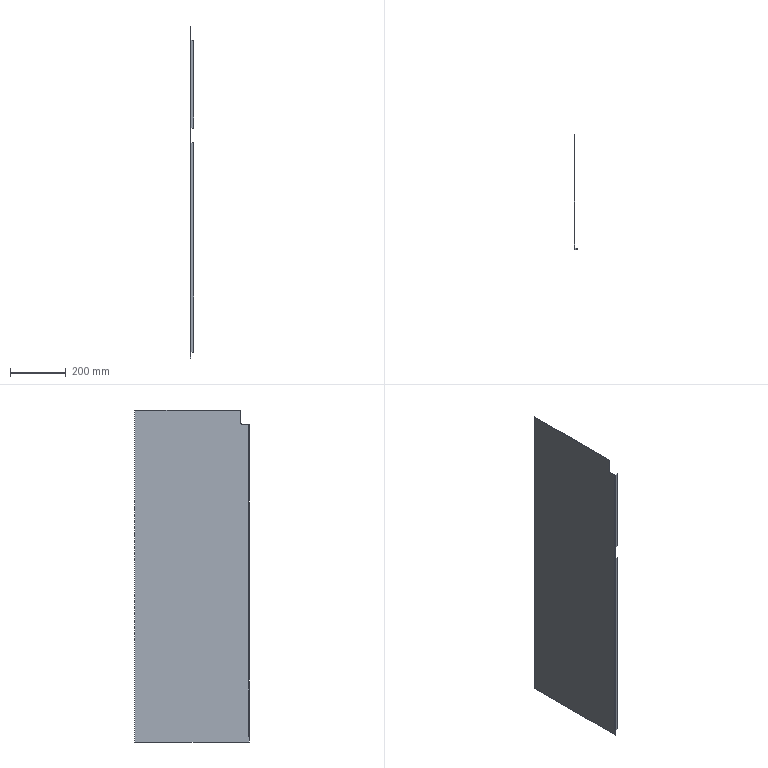Part | SolidWorks | 1 solid | 28 faces | box 12 x 410 x 1188 mm | volume 991648 mm3 | plane 25 | cylinder 3 | commonest cylinder face diameters 0.2 x1 4.2 x1 10 x1
STEP:
#1=CARTESIAN_POINT('',(10.,-205.,-573.25));
#2=VERTEX_POINT('',#1);
#3=CARTESIAN_POINT('',(10.,-205.,176.75));
#4=VERTEX_POINT('',#3);
#5=CARTESIAN_POINT('',(10.,-205.,0.));
#6=DIRECTION('',(0.,0.,1.));
#7=VECTOR('',#6,1000.);
#8=LINE('',#5,#7);
#9=EDGE_CURVE('',#2,#4,#8,.T.);
#10=ORIENTED_EDGE('',*,*,#9,.T.);
#11=CARTESIAN_POINT('',(0.1,-205.,176.75));
#12=VERTEX_POINT('',#11);
#13=CARTESIAN_POINT('',(0.,-205.,176.75));
#14=DIRECTION('',(1.,0.,0.));
#15=VECTOR('',#14,1000.);
#16=LINE('',#13,#15);
#17=EDGE_CURVE('',#12,#4,#16,.T.);
#18=ORIENTED_EDGE('',*,*,#17,.F.);
#19=CARTESIAN_POINT('',(0.1,-205.,-573.25));
#20=VERTEX_POINT('',#19);
#21=CARTESIAN_POINT('',(0.1,-205.,543.25));
#22=DIRECTION('',(0.,0.,1.));
#23=VECTOR('',#22,1000.);
#24=LINE('',#21,#23);
#25=EDGE_CURVE('',#20,#12,#24,.T.);
#26=ORIENTED_EDGE('',*,*,#25,.F.);
#27=CARTESIAN_POINT('',(0.,-205.,-573.25));
#28=DIRECTION('',(1.,0.,0.));
#29=VECTOR('',#28,1000.);
#30=LINE('',#27,#29);
#31=EDGE_CURVE('',#20,#2,#30,.T.);
#32=ORIENTED_EDGE('',*,*,#31,.T.);
#33=EDGE_LOOP('',(#10,#18,#26,#32));
#34=FACE_OUTER_BOUND('',#33,.T.);
#35=CARTESIAN_POINT('',(0.,-205.,0.));
#36=DIRECTION('',(0.,1.,0.));
#37=DIRECTION('',(-1.,0.,0.));
#38=AXIS2_PLACEMENT_3D('',#35,#36,#37);
#39=PLANE('',#38);
#40=ADVANCED_FACE('',(#34),#39,.F.);
#41=CARTESIAN_POINT('',(10.,-203.,176.75));
#42=VERTEX_POINT('',#41);
#43=CARTESIAN_POINT('',(0.1,-203.,176.75));
#44=VERTEX_POINT('',#43);
#45=CARTESIAN_POINT('',(0.,-203.,176.75));
#46=DIRECTION('',(-1.,0.,0.));
#47=VECTOR('',#46,1000.);
#48=LINE('',#45,#47);
#49=EDGE_CURVE('',#42,#44,#48,.T.);
#50=ORIENTED_EDGE('',*,*,#49,.F.);
#51=CARTESIAN_POINT('',(10.,-203.,-573.25));
#52=VERTEX_POINT('',#51);
#53=CARTESIAN_POINT('',(10.,-203.,543.25));
#54=DIRECTION('',(0.,0.,1.));
#55=VECTOR('',#54,1000.);
#56=LINE('',#53,#55);
#57=EDGE_CURVE('',#52,#42,#56,.T.);
#58=ORIENTED_EDGE('',*,*,#57,.F.);
#59=CARTESIAN_POINT('',(0.1,-203.,-573.25));
#60=VERTEX_POINT('',#59);
#61=CARTESIAN_POINT('',(10.,-203.,-573.25));
#62=DIRECTION('',(1.,0.,0.));
#63=VECTOR('',#62,1000.);
#64=LINE('',#61,#63);
#65=EDGE_CURVE('',#60,#52,#64,.T.);
#66=ORIENTED_EDGE('',*,*,#65,.F.);
#67=CARTESIAN_POINT('',(0.1,-203.,543.25));
#68=DIRECTION('',(0.,0.,-1.));
#69=VECTOR('',#68,1000.);
#70=LINE('',#67,#69);
#71=EDGE_CURVE('',#44,#60,#70,.T.);
#72=ORIENTED_EDGE('',*,*,#71,.F.);
#73=EDGE_LOOP('',(#50,#58,#66,#72));
#74=FACE_OUTER_BOUND('',#73,.T.);
#75=CARTESIAN_POINT('',(0.,-203.,0.));
#76=DIRECTION('',(0.,1.,0.));
#77=DIRECTION('',(-1.,0.,0.));
#78=AXIS2_PLACEMENT_3D('',#75,#76,#77);
#79=PLANE('',#78);
#80=ADVANCED_FACE('',(#74),#79,.T.);
#81=ORIENTED_EDGE('',*,*,#57,.T.);
#82=CARTESIAN_POINT('',(10.,-205.001,176.75));
#83=DIRECTION('',(0.,1.,0.));
#84=VECTOR('',#83,1000.);
#85=LINE('',#82,#84);
#86=EDGE_CURVE('',#4,#42,#85,.T.);
#87=ORIENTED_EDGE('',*,*,#86,.F.);
#88=ORIENTED_EDGE('',*,*,#9,.F.);
#89=CARTESIAN_POINT('',(10.,-205.,-573.25));
#90=DIRECTION('',(0.,1.,0.));
#91=VECTOR('',#90,1000.);
#92=LINE('',#89,#91);
#93=EDGE_CURVE('',#2,#52,#92,.T.);
#94=ORIENTED_EDGE('',*,*,#93,.T.);
#95=EDGE_LOOP('',(#81,#87,#88,#94));
#96=FACE_OUTER_BOUND('',#95,.T.);
#97=CARTESIAN_POINT('',(10.,-205.,543.25));
#98=DIRECTION('',(-1.,0.,0.));
#99=DIRECTION('',(0.,-1.,0.));
#100=AXIS2_PLACEMENT_3D('',#97,#98,#99);
#101=PLANE('',#100);
#102=ADVANCED_FACE('',(#96),#101,.F.);
#103=CARTESIAN_POINT('',(0.,-205.,-574.25));
#104=VERTEX_POINT('',#103);
#105=CARTESIAN_POINT('',(0.,-205.,-594.25));
#106=VERTEX_POINT('',#105);
#107=CARTESIAN_POINT('',(0.,-205.,-594.25));
#108=DIRECTION('',(0.,0.,-1.));
#109=VECTOR('',#108,1000.);
#110=LINE('',#107,#109);
#111=EDGE_CURVE('',#104,#106,#110,.T.);
#112=ORIENTED_EDGE('',*,*,#111,.F.);
#113=CARTESIAN_POINT('',(-2.,-205.,-574.25));
#114=VERTEX_POINT('',#113);
#115=CARTESIAN_POINT('',(0.,-205.,-574.25));
#116=DIRECTION('',(-1.,0.,0.));
#117=VECTOR('',#116,1000.);
#118=LINE('',#115,#117);
#119=EDGE_CURVE('',#104,#114,#118,.T.);
#120=ORIENTED_EDGE('',*,*,#119,.T.);
#121=CARTESIAN_POINT('',(-2.,-205.,-594.25));
#122=VERTEX_POINT('',#121);
#123=CARTESIAN_POINT('',(-2.,-205.,-594.25));
#124=DIRECTION('',(0.,0.,-1.));
#125=VECTOR('',#124,1000.);
#126=LINE('',#123,#125);
#127=EDGE_CURVE('',#114,#122,#126,.T.);
#128=ORIENTED_EDGE('',*,*,#127,.T.);
#129=CARTESIAN_POINT('',(-2.,-205.,-594.25));
#130=DIRECTION('',(1.,0.,0.));
#131=VECTOR('',#130,1000.);
#132=LINE('',#129,#131);
#133=EDGE_CURVE('',#122,#106,#132,.T.);
#134=ORIENTED_EDGE('',*,*,#133,.T.);
#135=EDGE_LOOP('',(#112,#120,#128,#134));
#136=FACE_OUTER_BOUND('',#135,.T.);
#137=CARTESIAN_POINT('',(-2.,-205.,-594.25));
#138=DIRECTION('',(0.,-1.,0.));
#139=DIRECTION('',(0.,0.,-1.));
#140=AXIS2_PLACEMENT_3D('',#137,#138,#139);
#141=PLANE('',#140);
#142=ADVANCED_FACE('',(#136),#141,.T.);
#143=CARTESIAN_POINT('',(-2.,-179.,543.25));
#144=VERTEX_POINT('',#143);
#145=CARTESIAN_POINT('',(-2.,-202.9,543.25));
#146=VERTEX_POINT('',#145);
#147=CARTESIAN_POINT('',(-2.,0.,543.25));
#148=DIRECTION('',(0.,-1.,0.));
#149=VECTOR('',#148,1000.);
#150=LINE('',#147,#149);
#151=EDGE_CURVE('',#144,#146,#150,.T.);
#152=ORIENTED_EDGE('',*,*,#151,.F.);
#153=CARTESIAN_POINT('',(-2.,-174.,548.25));
#154=VERTEX_POINT('',#153);
#155=CARTESIAN_POINT('',(-2.,-179.,548.25));
#156=DIRECTION('',(-1.,0.,0.));
#157=DIRECTION('',(0.,0.,-1.));
#158=AXIS2_PLACEMENT_3D('',#155,#156,#157);
#159=CIRCLE('',#158,5.);
#160=EDGE_CURVE('',#154,#144,#159,.T.);
#161=ORIENTED_EDGE('',*,*,#160,.F.);
#162=CARTESIAN_POINT('',(-2.,-174.,594.25));
#163=VERTEX_POINT('',#162);
#164=CARTESIAN_POINT('',(-2.,-174.,598.25));
#165=DIRECTION('',(0.,0.,-1.));
#166=VECTOR('',#165,1000.);
#167=LINE('',#164,#166);
#168=EDGE_CURVE('',#163,#154,#167,.T.);
#169=ORIENTED_EDGE('',*,*,#168,.F.);
#170=CARTESIAN_POINT('',(-2.,205.,594.25));
#171=VERTEX_POINT('',#170);
#172=CARTESIAN_POINT('',(-2.,-205.,594.25));
#173=DIRECTION('',(0.,-1.,0.));
#174=VECTOR('',#173,1000.);
#175=LINE('',#172,#174);
#176=EDGE_CURVE('',#171,#163,#175,.T.);
#177=ORIENTED_EDGE('',*,*,#176,.F.);
#178=CARTESIAN_POINT('',(-2.,205.,-594.25));
#179=VERTEX_POINT('',#178);
#180=CARTESIAN_POINT('',(-2.,205.,-594.25));
#181=DIRECTION('',(0.,0.,1.));
#182=VECTOR('',#181,1000.);
#183=LINE('',#180,#182);
#184=EDGE_CURVE('',#179,#171,#183,.T.);
#185=ORIENTED_EDGE('',*,*,#184,.F.);
#186=CARTESIAN_POINT('',(-2.,-205.,-594.25));
#187=DIRECTION('',(0.,1.,0.));
#188=VECTOR('',#187,1000.);
#189=LINE('',#186,#188);
#190=EDGE_CURVE('',#122,#179,#189,.T.);
#191=ORIENTED_EDGE('',*,*,#190,.F.);
#192=ORIENTED_EDGE('',*,*,#127,.F.);
#193=CARTESIAN_POINT('',(-2.,-201.9,-574.25));
#194=VERTEX_POINT('',#193);
#195=CARTESIAN_POINT('',(-2.,0.,-574.25));
#196=DIRECTION('',(0.,-1.,0.));
#197=VECTOR('',#196,1000.);
#198=LINE('',#195,#197);
#199=EDGE_CURVE('',#194,#114,#198,.T.);
#200=ORIENTED_EDGE('',*,*,#199,.F.);
#201=CARTESIAN_POINT('',(-2.,-201.9,-573.25));
#202=VERTEX_POINT('',#201);
#203=CARTESIAN_POINT('',(-2.,-201.9,0.));
#204=DIRECTION('',(0.,0.,-1.));
#205=VECTOR('',#204,1000.);
#206=LINE('',#203,#205);
#207=EDGE_CURVE('',#202,#194,#206,.T.);
#208=ORIENTED_EDGE('',*,*,#207,.F.);
#209=CARTESIAN_POINT('',(-2.,-202.9,-573.25));
#210=VERTEX_POINT('',#209);
#211=CARTESIAN_POINT('',(-2.,0.,-573.25));
#212=DIRECTION('',(0.,1.,0.));
#213=VECTOR('',#212,1000.);
#214=LINE('',#211,#213);
#215=EDGE_CURVE('',#210,#202,#214,.T.);
#216=ORIENTED_EDGE('',*,*,#215,.F.);
#217=CARTESIAN_POINT('',(-2.,-202.9,-573.25));
#218=DIRECTION('',(0.,0.,1.));
#219=VECTOR('',#218,1000.);
#220=LINE('',#217,#219);
#221=EDGE_CURVE('',#210,#146,#220,.T.);
#222=ORIENTED_EDGE('',*,*,#221,.T.);
#223=EDGE_LOOP('',(#152,#161,#169,#177,#185,#191,#192,#200,#208,#216,#222));
#224=FACE_OUTER_BOUND('',#223,.T.);
#225=CARTESIAN_POINT('',(-2.,0.,0.));
#226=DIRECTION('',(1.,0.,0.));
#227=DIRECTION('',(0.,0.,-1.));
#228=AXIS2_PLACEMENT_3D('',#225,#226,#227);
#229=PLANE('',#228);
#230=ADVANCED_FACE('',(#224),#229,.F.);
#231=CARTESIAN_POINT('',(0.,-174.,548.25));
#232=VERTEX_POINT('',#231);
#233=CARTESIAN_POINT('',(0.,-179.,543.25));
#234=VERTEX_POINT('',#233);
#235=CARTESIAN_POINT('',(0.,-179.,548.25));
#236=DIRECTION('',(-1.,0.,0.));
#237=DIRECTION('',(0.,0.,-1.));
#238=AXIS2_PLACEMENT_3D('',#235,#236,#237);
#239=CIRCLE('',#238,5.);
#240=EDGE_CURVE('',#232,#234,#239,.T.);
#241=ORIENTED_EDGE('',*,*,#240,.T.);
#242=CARTESIAN_POINT('',(0.,-202.9,543.25));
#243=VERTEX_POINT('',#242);
#244=CARTESIAN_POINT('',(0.,-202.9,543.25));
#245=DIRECTION('',(0.,1.,0.));
#246=VECTOR('',#245,1000.);
#247=LINE('',#244,#246);
#248=EDGE_CURVE('',#243,#234,#247,.T.);
#249=ORIENTED_EDGE('',*,*,#248,.F.);
#250=CARTESIAN_POINT('',(0.,-202.9,-573.25));
#251=VERTEX_POINT('',#250);
#252=CARTESIAN_POINT('',(0.,-202.9,-573.25));
#253=DIRECTION('',(0.,0.,1.));
#254=VECTOR('',#253,1000.);
#255=LINE('',#252,#254);
#256=EDGE_CURVE('',#251,#243,#255,.T.);
#257=ORIENTED_EDGE('',*,*,#256,.F.);
#258=CARTESIAN_POINT('',(0.,-201.9,-573.25));
#259=VERTEX_POINT('',#258);
#260=CARTESIAN_POINT('',(0.,-201.9,-573.25));
#261=DIRECTION('',(0.,-1.,0.));
#262=VECTOR('',#261,1000.);
#263=LINE('',#260,#262);
#264=EDGE_CURVE('',#259,#251,#263,.T.);
#265=ORIENTED_EDGE('',*,*,#264,.F.);
#266=CARTESIAN_POINT('',(0.,-201.9,-574.25));
#267=VERTEX_POINT('',#266);
#268=CARTESIAN_POINT('',(0.,-201.9,-574.25));
#269=DIRECTION('',(0.,0.,1.));
#270=VECTOR('',#269,1000.);
#271=LINE('',#268,#270);
#272=EDGE_CURVE('',#267,#259,#271,.T.);
#273=ORIENTED_EDGE('',*,*,#272,.F.);
#274=CARTESIAN_POINT('',(0.,-205.,-574.25));
#275=DIRECTION('',(0.,1.,0.));
#276=VECTOR('',#275,1000.);
#277=LINE('',#274,#276);
#278=EDGE_CURVE('',#104,#267,#277,.T.);
#279=ORIENTED_EDGE('',*,*,#278,.F.);
#280=ORIENTED_EDGE('',*,*,#111,.T.);
#281=CARTESIAN_POINT('',(0.,205.,-594.25));
#282=VERTEX_POINT('',#281);
#283=CARTESIAN_POINT('',(0.,-205.,-594.25));
#284=DIRECTION('',(0.,1.,0.));
#285=VECTOR('',#284,1000.);
#286=LINE('',#283,#285);
#287=EDGE_CURVE('',#106,#282,#286,.T.);
#288=ORIENTED_EDGE('',*,*,#287,.T.);
#289=CARTESIAN_POINT('',(0.,205.,594.25));
#290=VERTEX_POINT('',#289);
#291=CARTESIAN_POINT('',(0.,205.,-594.25));
#292=DIRECTION('',(0.,0.,1.));
#293=VECTOR('',#292,1000.);
#294=LINE('',#291,#293);
#295=EDGE_CURVE('',#282,#290,#294,.T.);
#296=ORIENTED_EDGE('',*,*,#295,.T.);
#297=CARTESIAN_POINT('',(0.,-174.,594.25));
#298=VERTEX_POINT('',#297);
#299=CARTESIAN_POINT('',(0.,-205.,594.25));
#300=DIRECTION('',(0.,-1.,0.));
#301=VECTOR('',#300,1000.);
#302=LINE('',#299,#301);
#303=EDGE_CURVE('',#290,#298,#302,.T.);
#304=ORIENTED_EDGE('',*,*,#303,.T.);
#305=CARTESIAN_POINT('',(0.,-174.,598.25));
#306=DIRECTION('',(0.,0.,-1.));
#307=VECTOR('',#306,1000.);
#308=LINE('',#305,#307);
#309=EDGE_CURVE('',#298,#232,#308,.T.);
#310=ORIENTED_EDGE('',*,*,#309,.T.);
#311=EDGE_LOOP('',(#241,#249,#257,#265,#273,#279,#280,#288,#296,#304,#310));
#312=FACE_OUTER_BOUND('',#311,.T.);
#313=CARTESIAN_POINT('',(0.,0.,0.));
#314=DIRECTION('',(1.,0.,0.));
#315=DIRECTION('',(0.,0.,-1.));
#316=AXIS2_PLACEMENT_3D('',#313,#314,#315);
#317=PLANE('',#316);
#318=ADVANCED_FACE('',(#312),#317,.T.);
#319=CARTESIAN_POINT('',(10.001,-174.,594.25));
#320=DIRECTION('',(1.,0.,0.));
#321=VECTOR('',#320,1000.);
#322=LINE('',#319,#321);
#323=EDGE_CURVE('',#163,#298,#322,.T.);
#324=ORIENTED_EDGE('',*,*,#323,.T.);
#325=ORIENTED_EDGE('',*,*,#303,.F.);
#326=CARTESIAN_POINT('',(-2.,205.,594.25));
#327=DIRECTION('',(1.,0.,0.));
#328=VECTOR('',#327,1000.);
#329=LINE('',#326,#328);
#330=EDGE_CURVE('',#171,#290,#329,.T.);
#331=ORIENTED_EDGE('',*,*,#330,.F.);
#332=ORIENTED_EDGE('',*,*,#176,.T.);
#333=EDGE_LOOP('',(#324,#325,#331,#332));
#334=FACE_OUTER_BOUND('',#333,.T.);
#335=CARTESIAN_POINT('',(-2.,-205.,594.25));
#336=DIRECTION('',(0.,0.,1.));
#337=DIRECTION('',(1.,0.,0.));
#338=AXIS2_PLACEMENT_3D('',#335,#336,#337);
#339=PLANE('',#338);
#340=ADVANCED_FACE('',(#334),#339,.T.);
#341=ORIENTED_EDGE('',*,*,#295,.F.);
#342=CARTESIAN_POINT('',(-2.,205.,-594.25));
#343=DIRECTION('',(1.,0.,0.));
#344=VECTOR('',#343,1000.);
#345=LINE('',#342,#344);
#346=EDGE_CURVE('',#179,#282,#345,.T.);
#347=ORIENTED_EDGE('',*,*,#346,.F.);
#348=ORIENTED_EDGE('',*,*,#184,.T.);
#349=ORIENTED_EDGE('',*,*,#330,.T.);
#350=EDGE_LOOP('',(#341,#347,#348,#349));
#351=FACE_OUTER_BOUND('',#350,.T.);
#352=CARTESIAN_POINT('',(-2.,205.,-594.25));
#353=DIRECTION('',(0.,1.,0.));
#354=DIRECTION('',(0.,0.,1.));
#355=AXIS2_PLACEMENT_3D('',#352,#353,#354);
#356=PLANE('',#355);
#357=ADVANCED_FACE('',(#351),#356,.T.);
#358=ORIENTED_EDGE('',*,*,#287,.F.);
#359=ORIENTED_EDGE('',*,*,#133,.F.);
#360=ORIENTED_EDGE('',*,*,#190,.T.);
#361=ORIENTED_EDGE('',*,*,#346,.T.);
#362=EDGE_LOOP('',(#358,#359,#360,#361));
#363=FACE_OUTER_BOUND('',#362,.T.);
#364=CARTESIAN_POINT('',(-2.,-205.,-594.25));
#365=DIRECTION('',(0.,0.,-1.));
#366=DIRECTION('',(-1.,0.,0.));
#367=AXIS2_PLACEMENT_3D('',#364,#365,#366);
#368=PLANE('',#367);
#369=ADVANCED_FACE('',(#363),#368,.T.);
#370=CARTESIAN_POINT('',(0.,-201.9,-574.25));
#371=DIRECTION('',(-1.,0.,0.));
#372=VECTOR('',#371,1000.);
#373=LINE('',#370,#372);
#374=EDGE_CURVE('',#267,#194,#373,.T.);
#375=ORIENTED_EDGE('',*,*,#374,.T.);
#376=ORIENTED_EDGE('',*,*,#199,.T.);
#377=ORIENTED_EDGE('',*,*,#119,.F.);
#378=ORIENTED_EDGE('',*,*,#278,.T.);
#379=EDGE_LOOP('',(#375,#376,#377,#378));
#380=FACE_OUTER_BOUND('',#379,.T.);
#381=CARTESIAN_POINT('',(0.,-205.,-574.25));
#382=DIRECTION('',(0.,0.,1.));
#383=DIRECTION('',(1.,0.,0.));
#384=AXIS2_PLACEMENT_3D('',#381,#382,#383);
#385=PLANE('',#384);
#386=ADVANCED_FACE('',(#380),#385,.T.);
#387=CARTESIAN_POINT('',(0.,-201.9,-573.25));
#388=DIRECTION('',(-1.,0.,0.));
#389=VECTOR('',#388,1000.);
#390=LINE('',#387,#389);
#391=EDGE_CURVE('',#259,#202,#390,.T.);
#392=ORIENTED_EDGE('',*,*,#391,.T.);
#393=ORIENTED_EDGE('',*,*,#207,.T.);
#394=ORIENTED_EDGE('',*,*,#374,.F.);
#395=ORIENTED_EDGE('',*,*,#272,.T.);
#396=EDGE_LOOP('',(#392,#393,#394,#395));
#397=FACE_OUTER_BOUND('',#396,.T.);
#398=CARTESIAN_POINT('',(0.,-201.9,-574.25));
#399=DIRECTION('',(0.,-1.,0.));
#400=DIRECTION('',(0.,0.,-1.));
#401=AXIS2_PLACEMENT_3D('',#398,#399,#400);
#402=PLANE('',#401);
#403=ADVANCED_FACE('',(#397),#402,.T.);
#404=CARTESIAN_POINT('',(0.,-202.9,-573.25));
#405=DIRECTION('',(-1.,0.,0.));
#406=VECTOR('',#405,1000.);
#407=LINE('',#404,#406);
#408=EDGE_CURVE('',#251,#210,#407,.T.);
#409=ORIENTED_EDGE('',*,*,#408,.T.);
#410=ORIENTED_EDGE('',*,*,#215,.T.);
#411=ORIENTED_EDGE('',*,*,#391,.F.);
#412=ORIENTED_EDGE('',*,*,#264,.T.);
#413=EDGE_LOOP('',(#409,#410,#411,#412));
#414=FACE_OUTER_BOUND('',#413,.T.);
#415=CARTESIAN_POINT('',(0.,-201.9,-573.25));
#416=DIRECTION('',(0.,0.,-1.));
#417=DIRECTION('',(-1.,0.,0.));
#418=AXIS2_PLACEMENT_3D('',#415,#416,#417);
#419=PLANE('',#418);
#420=ADVANCED_FACE('',(#414),#419,.T.);
#421=ORIENTED_EDGE('',*,*,#248,.T.);
#422=CARTESIAN_POINT('',(10.001,-179.,543.25));
#423=DIRECTION('',(-1.,0.,0.));
#424=VECTOR('',#423,1000.);
#425=LINE('',#422,#424);
#426=EDGE_CURVE('',#234,#144,#425,.T.);
#427=ORIENTED_EDGE('',*,*,#426,.T.);
#428=ORIENTED_EDGE('',*,*,#151,.T.);
#429=CARTESIAN_POINT('',(0.,-202.9,543.25));
#430=DIRECTION('',(-1.,0.,0.));
#431=VECTOR('',#430,1000.);
#432=LINE('',#429,#431);
#433=EDGE_CURVE('',#243,#146,#432,.T.);
#434=ORIENTED_EDGE('',*,*,#433,.F.);
#435=EDGE_LOOP('',(#421,#427,#428,#434));
#436=FACE_OUTER_BOUND('',#435,.T.);
#437=CARTESIAN_POINT('',(0.,-202.9,543.25));
#438=DIRECTION('',(0.,0.,1.));
#439=DIRECTION('',(1.,0.,0.));
#440=AXIS2_PLACEMENT_3D('',#437,#438,#439);
#441=PLANE('',#440);
#442=ADVANCED_FACE('',(#436),#441,.T.);
#443=CARTESIAN_POINT('',(0.1,-203.,543.25));
#444=VERTEX_POINT('',#443);
#445=CARTESIAN_POINT('',(0.1,-205.,543.25));
#446=VERTEX_POINT('',#445);
#447=CARTESIAN_POINT('',(0.1,-205.,543.25));
#448=DIRECTION('',(0.,-1.,0.));
#449=VECTOR('',#448,1000.);
#450=LINE('',#447,#449);
#451=EDGE_CURVE('',#444,#446,#450,.T.);
#452=ORIENTED_EDGE('',*,*,#451,.F.);
#453=CARTESIAN_POINT('',(0.1,-202.9,543.25));
#454=DIRECTION('',(0.,0.,1.));
#455=DIRECTION('',(-1.,0.,0.));
#456=AXIS2_PLACEMENT_3D('',#453,#454,#455);
#457=CIRCLE('',#456,0.1);
#458=EDGE_CURVE('',#243,#444,#457,.T.);
#459=ORIENTED_EDGE('',*,*,#458,.F.);
#460=ORIENTED_EDGE('',*,*,#433,.T.);
#461=CARTESIAN_POINT('',(0.1,-202.9,543.25));
#462=DIRECTION('',(0.,0.,1.));
#463=DIRECTION('',(-1.,0.,0.));
#464=AXIS2_PLACEMENT_3D('',#461,#462,#463);
#465=CIRCLE('',#464,2.1);
#466=EDGE_CURVE('',#146,#446,#465,.T.);
#467=ORIENTED_EDGE('',*,*,#466,.T.);
#468=EDGE_LOOP('',(#452,#459,#460,#467));
#469=FACE_OUTER_BOUND('',#468,.T.);
#470=CARTESIAN_POINT('',(0.1,-202.9,543.25));
#471=DIRECTION('',(0.,0.,1.));
#472=DIRECTION('',(1.,0.,0.));
#473=AXIS2_PLACEMENT_3D('',#470,#471,#472);
#474=PLANE('',#473);
#475=ADVANCED_FACE('',(#469),#474,.T.);
#476=CARTESIAN_POINT('',(0.1,-202.9,-573.25));
#477=DIRECTION('',(0.,0.,-1.));
#478=DIRECTION('',(-1.,0.,0.));
#479=AXIS2_PLACEMENT_3D('',#476,#477,#478);
#480=CIRCLE('',#479,0.1);
#481=EDGE_CURVE('',#60,#251,#480,.T.);
#482=ORIENTED_EDGE('',*,*,#481,.F.);
#483=CARTESIAN_POINT('',(0.1,-203.,-573.25));
#484=DIRECTION('',(0.,-1.,0.));
#485=VECTOR('',#484,1000.);
#486=LINE('',#483,#485);
#487=EDGE_CURVE('',#60,#20,#486,.T.);
#488=ORIENTED_EDGE('',*,*,#487,.T.);
#489=CARTESIAN_POINT('',(0.1,-202.9,-573.25));
#490=DIRECTION('',(0.,0.,-1.));
#491=DIRECTION('',(-1.,0.,0.));
#492=AXIS2_PLACEMENT_3D('',#489,#490,#491);
#493=CIRCLE('',#492,2.1);
#494=EDGE_CURVE('',#20,#210,#493,.T.);
#495=ORIENTED_EDGE('',*,*,#494,.T.);
#496=ORIENTED_EDGE('',*,*,#408,.F.);
#497=EDGE_LOOP('',(#482,#488,#495,#496));
#498=FACE_OUTER_BOUND('',#497,.T.);
#499=CARTESIAN_POINT('',(0.1,-202.9,-573.25));
#500=DIRECTION('',(0.,0.,1.));
#501=DIRECTION('',(1.,0.,0.));
#502=AXIS2_PLACEMENT_3D('',#499,#500,#501);
#503=PLANE('',#502);
#504=ADVANCED_FACE('',(#498),#503,.F.);
#505=CARTESIAN_POINT('',(0.,-204.998,176.75));
#506=VERTEX_POINT('',#505);
#507=CARTESIAN_POINT('',(0.1,-202.9,176.75));
#508=DIRECTION('',(0.,0.,-1.));
#509=DIRECTION('',(0.,1.,0.));
#510=AXIS2_PLACEMENT_3D('',#507,#508,#509);
#511=CIRCLE('',#510,2.1);
#512=EDGE_CURVE('',#12,#506,#511,.T.);
#513=ORIENTED_EDGE('',*,*,#512,.T.);
#514=CARTESIAN_POINT('',(0.,-204.998,228.75));
#515=VERTEX_POINT('',#514);
#516=CARTESIAN_POINT('',(0.,-204.998,-573.25));
#517=DIRECTION('',(0.,0.,1.));
#518=VECTOR('',#517,1000.);
#519=LINE('',#516,#518);
#520=EDGE_CURVE('',#506,#515,#519,.T.);
#521=ORIENTED_EDGE('',*,*,#520,.T.);
#522=CARTESIAN_POINT('',(0.1,-205.,228.75));
#523=VERTEX_POINT('',#522);
#524=CARTESIAN_POINT('',(0.1,-202.9,228.75));
#525=DIRECTION('',(0.,0.,1.));
#526=DIRECTION('',(0.,-1.,0.));
#527=AXIS2_PLACEMENT_3D('',#524,#525,#526);
#528=CIRCLE('',#527,2.1);
#529=EDGE_CURVE('',#515,#523,#528,.T.);
#530=ORIENTED_EDGE('',*,*,#529,.T.);
#531=CARTESIAN_POINT('',(0.1,-205.,543.25));
#532=DIRECTION('',(0.,0.,1.));
#533=VECTOR('',#532,1000.);
#534=LINE('',#531,#533);
#535=EDGE_CURVE('',#523,#446,#534,.T.);
#536=ORIENTED_EDGE('',*,*,#535,.T.);
#537=ORIENTED_EDGE('',*,*,#466,.F.);
#538=ORIENTED_EDGE('',*,*,#221,.F.);
#539=ORIENTED_EDGE('',*,*,#494,.F.);
#540=ORIENTED_EDGE('',*,*,#25,.T.);
#541=EDGE_LOOP('',(#513,#521,#530,#536,#537,#538,#539,#540));
#542=FACE_OUTER_BOUND('',#541,.T.);
#543=CARTESIAN_POINT('',(0.1,-202.9,-573.25));
#544=DIRECTION('',(0.,0.,-1.));
#545=DIRECTION('',(0.,-1.,0.));
#546=AXIS2_PLACEMENT_3D('',#543,#544,#545);
#547=CYLINDRICAL_SURFACE('',#546,2.1);
#548=ADVANCED_FACE('',(#542),#547,.T.);
#549=ORIENTED_EDGE('',*,*,#256,.T.);
#550=ORIENTED_EDGE('',*,*,#458,.T.);
#551=CARTESIAN_POINT('',(0.1,-203.,228.75));
#552=VERTEX_POINT('',#551);
#553=CARTESIAN_POINT('',(0.1,-203.,543.25));
#554=DIRECTION('',(0.,0.,-1.));
#555=VECTOR('',#554,1000.);
#556=LINE('',#553,#555);
#557=EDGE_CURVE('',#444,#552,#556,.T.);
#558=ORIENTED_EDGE('',*,*,#557,.T.);
#559=CARTESIAN_POINT('',(0.1,-203.,-573.25));
#560=DIRECTION('',(0.,0.,1.));
#561=VECTOR('',#560,1000.);
#562=LINE('',#559,#561);
#563=EDGE_CURVE('',#44,#552,#562,.T.);
#564=ORIENTED_EDGE('',*,*,#563,.F.);
#565=ORIENTED_EDGE('',*,*,#71,.T.);
#566=ORIENTED_EDGE('',*,*,#481,.T.);
#567=EDGE_LOOP('',(#549,#550,#558,#564,#565,#566));
#568=FACE_OUTER_BOUND('',#567,.T.);
#569=CARTESIAN_POINT('',(0.1,-202.9,-573.25));
#570=DIRECTION('',(0.,0.,-1.));
#571=DIRECTION('',(0.,-1.,0.));
#572=AXIS2_PLACEMENT_3D('',#569,#570,#571);
#573=CYLINDRICAL_SURFACE('',#572,0.1);
#574=ADVANCED_FACE('',(#568),#573,.F.);
#575=ORIENTED_EDGE('',*,*,#487,.F.);
#576=ORIENTED_EDGE('',*,*,#65,.T.);
#577=ORIENTED_EDGE('',*,*,#93,.F.);
#578=ORIENTED_EDGE('',*,*,#31,.F.);
#579=EDGE_LOOP('',(#575,#576,#577,#578));
#580=FACE_OUTER_BOUND('',#579,.T.);
#581=CARTESIAN_POINT('',(10.,-205.,-573.25));
#582=DIRECTION('',(0.,0.,1.));
#583=DIRECTION('',(1.,0.,0.));
#584=AXIS2_PLACEMENT_3D('',#581,#582,#583);
#585=PLANE('',#584);
#586=ADVANCED_FACE('',(#580),#585,.F.);
#587=ORIENTED_EDGE('',*,*,#451,.T.);
#588=CARTESIAN_POINT('',(10.,-205.,543.25));
#589=VERTEX_POINT('',#588);
#590=CARTESIAN_POINT('',(0.,-205.,543.25));
#591=DIRECTION('',(-1.,0.,0.));
#592=VECTOR('',#591,1000.);
#593=LINE('',#590,#592);
#594=EDGE_CURVE('',#589,#446,#593,.T.);
#595=ORIENTED_EDGE('',*,*,#594,.F.);
#596=CARTESIAN_POINT('',(10.,-203.,543.25));
#597=VERTEX_POINT('',#596);
#598=CARTESIAN_POINT('',(10.,-205.,543.25));
#599=DIRECTION('',(0.,1.,0.));
#600=VECTOR('',#599,1000.);
#601=LINE('',#598,#600);
#602=EDGE_CURVE('',#589,#597,#601,.T.);
#603=ORIENTED_EDGE('',*,*,#602,.T.);
#604=CARTESIAN_POINT('',(0.,-203.,543.25));
#605=DIRECTION('',(-1.,0.,0.));
#606=VECTOR('',#605,1000.);
#607=LINE('',#604,#606);
#608=EDGE_CURVE('',#597,#444,#607,.T.);
#609=ORIENTED_EDGE('',*,*,#608,.T.);
#610=EDGE_LOOP('',(#587,#595,#603,#609));
#611=FACE_OUTER_BOUND('',#610,.T.);
#612=CARTESIAN_POINT('',(0.,-205.,543.25));
#613=DIRECTION('',(0.,0.,-1.));
#614=DIRECTION('',(0.,1.,0.));
#615=AXIS2_PLACEMENT_3D('',#612,#613,#614);
#616=PLANE('',#615);
#617=ADVANCED_FACE('',(#611),#616,.F.);
#618=ORIENTED_EDGE('',*,*,#535,.F.);
#619=CARTESIAN_POINT('',(10.,-205.,228.75));
#620=VERTEX_POINT('',#619);
#621=CARTESIAN_POINT('',(0.,-205.,228.75));
#622=DIRECTION('',(-1.,0.,0.));
#623=VECTOR('',#622,1000.);
#624=LINE('',#621,#623);
#625=EDGE_CURVE('',#620,#523,#624,.T.);
#626=ORIENTED_EDGE('',*,*,#625,.F.);
#627=CARTESIAN_POINT('',(10.,-205.,0.));
#628=DIRECTION('',(0.,0.,1.));
#629=VECTOR('',#628,1000.);
#630=LINE('',#627,#629);
#631=EDGE_CURVE('',#620,#589,#630,.T.);
#632=ORIENTED_EDGE('',*,*,#631,.T.);
#633=ORIENTED_EDGE('',*,*,#594,.T.);
#634=EDGE_LOOP('',(#618,#626,#632,#633));
#635=FACE_OUTER_BOUND('',#634,.T.);
#636=CARTESIAN_POINT('',(0.,-205.,0.));
#637=DIRECTION('',(0.,1.,0.));
#638=DIRECTION('',(-1.,0.,0.));
#639=AXIS2_PLACEMENT_3D('',#636,#637,#638);
#640=PLANE('',#639);
#641=ADVANCED_FACE('',(#635),#640,.F.);
#642=CARTESIAN_POINT('',(10.,-203.,228.75));
#643=VERTEX_POINT('',#642);
#644=CARTESIAN_POINT('',(0.,-203.,228.75));
#645=DIRECTION('',(1.,0.,0.));
#646=VECTOR('',#645,1000.);
#647=LINE('',#644,#646);
#648=EDGE_CURVE('',#552,#643,#647,.T.);
#649=ORIENTED_EDGE('',*,*,#648,.F.);
#650=ORIENTED_EDGE('',*,*,#557,.F.);
#651=ORIENTED_EDGE('',*,*,#608,.F.);
#652=CARTESIAN_POINT('',(10.,-203.,543.25));
#653=DIRECTION('',(0.,0.,1.));
#654=VECTOR('',#653,1000.);
#655=LINE('',#652,#654);
#656=EDGE_CURVE('',#643,#597,#655,.T.);
#657=ORIENTED_EDGE('',*,*,#656,.F.);
#658=EDGE_LOOP('',(#649,#650,#651,#657));
#659=FACE_OUTER_BOUND('',#658,.T.);
#660=CARTESIAN_POINT('',(0.,-203.,0.));
#661=DIRECTION('',(0.,1.,0.));
#662=DIRECTION('',(-1.,0.,0.));
#663=AXIS2_PLACEMENT_3D('',#660,#661,#662);
#664=PLANE('',#663);
#665=ADVANCED_FACE('',(#659),#664,.T.);
#666=ORIENTED_EDGE('',*,*,#631,.F.);
#667=CARTESIAN_POINT('',(10.,-205.001,228.75));
#668=DIRECTION('',(0.,-1.,0.));
#669=VECTOR('',#668,1000.);
#670=LINE('',#667,#669);
#671=EDGE_CURVE('',#643,#620,#670,.T.);
#672=ORIENTED_EDGE('',*,*,#671,.F.);
#673=ORIENTED_EDGE('',*,*,#656,.T.);
#674=ORIENTED_EDGE('',*,*,#602,.F.);
#675=EDGE_LOOP('',(#666,#672,#673,#674));
#676=FACE_OUTER_BOUND('',#675,.T.);
#677=CARTESIAN_POINT('',(10.,-205.,543.25));
#678=DIRECTION('',(-1.,0.,0.));
#679=DIRECTION('',(0.,-1.,0.));
#680=AXIS2_PLACEMENT_3D('',#677,#678,#679);
#681=PLANE('',#680);
#682=ADVANCED_FACE('',(#676),#681,.F.);
#683=ORIENTED_EDGE('',*,*,#563,.T.);
#684=CARTESIAN_POINT('',(0.,-203.,228.75));
#685=VERTEX_POINT('',#684);
#686=CARTESIAN_POINT('',(0.,-203.,228.75));
#687=DIRECTION('',(1.,0.,0.));
#688=VECTOR('',#687,1000.);
#689=LINE('',#686,#688);
#690=EDGE_CURVE('',#685,#552,#689,.T.);
#691=ORIENTED_EDGE('',*,*,#690,.F.);
#692=CARTESIAN_POINT('',(0.,-203.,176.75));
#693=VERTEX_POINT('',#692);
#694=CARTESIAN_POINT('',(0.,-203.,176.75));
#695=DIRECTION('',(0.,0.,1.));
#696=VECTOR('',#695,1000.);
#697=LINE('',#694,#696);
#698=EDGE_CURVE('',#693,#685,#697,.T.);
#699=ORIENTED_EDGE('',*,*,#698,.F.);
#700=CARTESIAN_POINT('',(0.,-203.,176.75));
#701=DIRECTION('',(-1.,0.,0.));
#702=VECTOR('',#701,1000.);
#703=LINE('',#700,#702);
#704=EDGE_CURVE('',#44,#693,#703,.T.);
#705=ORIENTED_EDGE('',*,*,#704,.F.);
#706=EDGE_LOOP('',(#683,#691,#699,#705));
#707=FACE_OUTER_BOUND('',#706,.T.);
#708=CARTESIAN_POINT('',(0.,-203.,0.));
#709=DIRECTION('',(0.,1.,0.));
#710=DIRECTION('',(-1.,0.,0.));
#711=AXIS2_PLACEMENT_3D('',#708,#709,#710);
#712=PLANE('',#711);
#713=ADVANCED_FACE('',(#707),#712,.F.);
#714=CARTESIAN_POINT('',(0.,-205.001,176.75));
#715=DIRECTION('',(0.,1.,0.));
#716=VECTOR('',#715,1000.);
#717=LINE('',#714,#716);
#718=EDGE_CURVE('',#506,#693,#717,.T.);
#719=ORIENTED_EDGE('',*,*,#718,.T.);
#720=ORIENTED_EDGE('',*,*,#698,.T.);
#721=CARTESIAN_POINT('',(0.,-205.001,228.75));
#722=DIRECTION('',(0.,1.,0.));
#723=VECTOR('',#722,1000.);
#724=LINE('',#721,#723);
#725=EDGE_CURVE('',#515,#685,#724,.T.);
#726=ORIENTED_EDGE('',*,*,#725,.F.);
#727=ORIENTED_EDGE('',*,*,#520,.F.);
#728=EDGE_LOOP('',(#719,#720,#726,#727));
#729=FACE_OUTER_BOUND('',#728,.T.);
#730=CARTESIAN_POINT('',(0.,-205.001,176.75));
#731=DIRECTION('',(-1.,0.,0.));
#732=DIRECTION('',(0.,-1.,0.));
#733=AXIS2_PLACEMENT_3D('',#730,#731,#732);
#734=PLANE('',#733);
#735=ADVANCED_FACE('',(#729),#734,.F.);
#736=ORIENTED_EDGE('',*,*,#17,.T.);
#737=ORIENTED_EDGE('',*,*,#86,.T.);
#738=ORIENTED_EDGE('',*,*,#49,.T.);
#739=ORIENTED_EDGE('',*,*,#704,.T.);
#740=ORIENTED_EDGE('',*,*,#718,.F.);
#741=ORIENTED_EDGE('',*,*,#512,.F.);
#742=EDGE_LOOP('',(#736,#737,#738,#739,#740,#741));
#743=FACE_OUTER_BOUND('',#742,.T.);
#744=CARTESIAN_POINT('',(0.,-205.001,176.75));
#745=DIRECTION('',(0.,0.,-1.));
#746=DIRECTION('',(0.,1.,0.));
#747=AXIS2_PLACEMENT_3D('',#744,#745,#746);
#748=PLANE('',#747);
#749=ADVANCED_FACE('',(#743),#748,.F.);
#750=ORIENTED_EDGE('',*,*,#725,.T.);
#751=ORIENTED_EDGE('',*,*,#690,.T.);
#752=ORIENTED_EDGE('',*,*,#648,.T.);
#753=ORIENTED_EDGE('',*,*,#671,.T.);
#754=ORIENTED_EDGE('',*,*,#625,.T.);
#755=ORIENTED_EDGE('',*,*,#529,.F.);
#756=EDGE_LOOP('',(#750,#751,#752,#753,#754,#755));
#757=FACE_OUTER_BOUND('',#756,.T.);
#758=CARTESIAN_POINT('',(0.,-205.001,228.75));
#759=DIRECTION('',(0.,0.,1.));
#760=DIRECTION('',(0.,-1.,0.));
#761=AXIS2_PLACEMENT_3D('',#758,#759,#760);
#762=PLANE('',#761);
#763=ADVANCED_FACE('',(#757),#762,.F.);
#764=CARTESIAN_POINT('',(10.001,-174.,548.25));
#765=DIRECTION('',(-1.,0.,0.));
#766=VECTOR('',#765,1000.);
#767=LINE('',#764,#766);
#768=EDGE_CURVE('',#232,#154,#767,.T.);
#769=ORIENTED_EDGE('',*,*,#768,.T.);
#770=ORIENTED_EDGE('',*,*,#160,.T.);
#771=ORIENTED_EDGE('',*,*,#426,.F.);
#772=ORIENTED_EDGE('',*,*,#240,.F.);
#773=EDGE_LOOP('',(#769,#770,#771,#772));
#774=FACE_OUTER_BOUND('',#773,.T.);
#775=CARTESIAN_POINT('',(10.001,-179.,548.25));
#776=DIRECTION('',(-1.,0.,0.));
#777=DIRECTION('',(0.,0.,1.));
#778=AXIS2_PLACEMENT_3D('',#775,#776,#777);
#779=CYLINDRICAL_SURFACE('',#778,5.);
#780=ADVANCED_FACE('',(#774),#779,.F.);
#781=ORIENTED_EDGE('',*,*,#323,.F.);
#782=ORIENTED_EDGE('',*,*,#168,.T.);
#783=ORIENTED_EDGE('',*,*,#768,.F.);
#784=ORIENTED_EDGE('',*,*,#309,.F.);
#785=EDGE_LOOP('',(#781,#782,#783,#784));
#786=FACE_OUTER_BOUND('',#785,.T.);
#787=CARTESIAN_POINT('',(10.001,-174.,598.25));
#788=DIRECTION('',(0.,1.,0.));
#789=DIRECTION('',(0.,0.,1.));
#790=AXIS2_PLACEMENT_3D('',#787,#788,#789);
#791=PLANE('',#790);
#792=ADVANCED_FACE('',(#786),#791,.F.);
#793=CLOSED_SHELL('',(#40,#80,#102,#142,#230,#318,#340,#357,#369,#386,#403,#420,#442,#475,#504,#548,#574,#586,#617,#641,#665,#682,#713,#735,#749,#763,#780,#792));
#794=MANIFOLD_SOLID_BREP('',#793);
#795=CARTESIAN_POINT('',(0.,0.,0.));
#796=DIRECTION('',(0.,0.,1.));
#797=DIRECTION('',(1.,0.,0.));
#798=AXIS2_PLACEMENT_3D('',#795,#796,#797);
#799=(LENGTH_UNIT()NAMED_UNIT(*)SI_UNIT(.MILLI.,.METRE.));
#800=UNCERTAINTY_MEASURE_WITH_UNIT(LENGTH_MEASURE(0.00001),#799,'','');
#801=(NAMED_UNIT(*)PLANE_ANGLE_UNIT()SI_UNIT($,.RADIAN.));
#802=(NAMED_UNIT(*)SI_UNIT($,.STERADIAN.)SOLID_ANGLE_UNIT());
#803=(GEOMETRIC_REPRESENTATION_CONTEXT(3)GLOBAL_UNCERTAINTY_ASSIGNED_CONTEXT((#800))GLOBAL_UNIT_ASSIGNED_CONTEXT((#799,#801,#802))REPRESENTATION_CONTEXT('',''));
#804=ADVANCED_BREP_SHAPE_REPRESENTATION('',(#794,#798),#803);